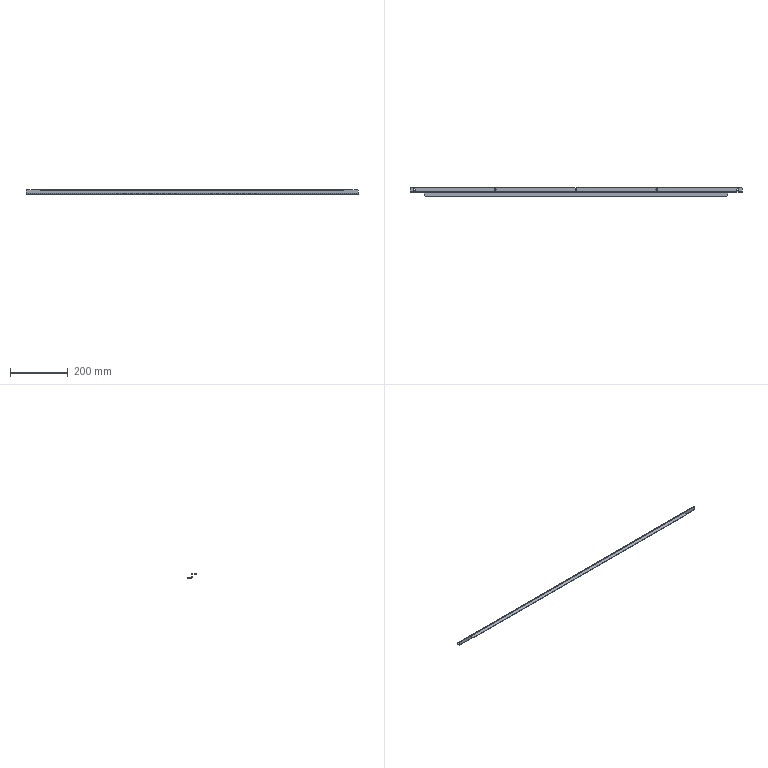Part | NX | features solid 2 | 1 solid | 38 faces | box 1150 x 30.5 x 15 mm | volume 70285 mm3 | plane 24 | cylinder 14 | commonest cylinder face diameters 6 x12 3 x2
STEP:
#1=CARTESIAN_POINT('',(-450.,-634.5,86.));
#2=VERTEX_POINT('',#1);
#3=CARTESIAN_POINT('',(-447.,-634.5,89.));
#4=VERTEX_POINT('',#3);
#5=CARTESIAN_POINT('',(-447.,-634.5,89.));
#6=DIRECTION('',(0.7071,0.,0.7071));
#7=VECTOR('',#6,1000.);
#8=LINE('',#5,#7);
#9=EDGE_CURVE('',#2,#4,#8,.T.);
#10=ORIENTED_EDGE('',*,*,#9,.F.);
#11=CARTESIAN_POINT('',(-450.,-636.,86.));
#12=VERTEX_POINT('',#11);
#13=CARTESIAN_POINT('',(-450.,-636.,86.));
#14=DIRECTION('',(0.,1.,0.));
#15=VECTOR('',#14,1000.);
#16=LINE('',#13,#15);
#17=EDGE_CURVE('',#12,#2,#16,.T.);
#18=ORIENTED_EDGE('',*,*,#17,.F.);
#19=CARTESIAN_POINT('',(-447.,-636.,89.));
#20=VERTEX_POINT('',#19);
#21=CARTESIAN_POINT('',(-448.5,-636.,87.5));
#22=DIRECTION('',(-0.7071,0.,-0.7071));
#23=VECTOR('',#22,1000.);
#24=LINE('',#21,#23);
#25=EDGE_CURVE('',#20,#12,#24,.T.);
#26=ORIENTED_EDGE('',*,*,#25,.F.);
#27=CARTESIAN_POINT('',(-447.,-636.,89.));
#28=DIRECTION('',(0.,-1.,0.));
#29=VECTOR('',#28,1000.);
#30=LINE('',#27,#29);
#31=EDGE_CURVE('',#4,#20,#30,.T.);
#32=ORIENTED_EDGE('',*,*,#31,.F.);
#33=EDGE_LOOP('',(#10,#18,#26,#32));
#34=FACE_BOUND('',#33,.T.);
#35=CARTESIAN_POINT('',(-447.,-636.,89.));
#36=DIRECTION('',(-0.7071,0.,0.7071));
#37=DIRECTION('',(0.,1.,0.));
#38=AXIS2_PLACEMENT_3D('',#35,#36,#37);
#39=PLANE('',#38);
#40=ADVANCED_FACE('',(#34),#39,.T.);
#41=CARTESIAN_POINT('',(-447.,-620.,75.5));
#42=VERTEX_POINT('',#41);
#43=CARTESIAN_POINT('',(-450.,-623.,75.5));
#44=VERTEX_POINT('',#43);
#45=CARTESIAN_POINT('',(-450.,-623.,75.5));
#46=DIRECTION('',(-0.7071,-0.7071,0.));
#47=VECTOR('',#46,1000.);
#48=LINE('',#45,#47);
#49=EDGE_CURVE('',#42,#44,#48,.T.);
#50=ORIENTED_EDGE('',*,*,#49,.F.);
#51=CARTESIAN_POINT('',(-447.,-620.,74.));
#52=VERTEX_POINT('',#51);
#53=CARTESIAN_POINT('',(-447.,-620.,74.));
#54=DIRECTION('',(0.,0.,1.));
#55=VECTOR('',#54,1000.);
#56=LINE('',#53,#55);
#57=EDGE_CURVE('',#52,#42,#56,.T.);
#58=ORIENTED_EDGE('',*,*,#57,.F.);
#59=CARTESIAN_POINT('',(-450.,-623.,74.));
#60=VERTEX_POINT('',#59);
#61=CARTESIAN_POINT('',(-456.5,-629.5,74.));
#62=DIRECTION('',(0.7071,0.7071,0.));
#63=VECTOR('',#62,1000.);
#64=LINE('',#61,#63);
#65=EDGE_CURVE('',#60,#52,#64,.T.);
#66=ORIENTED_EDGE('',*,*,#65,.F.);
#67=CARTESIAN_POINT('',(-450.,-623.,74.));
#68=DIRECTION('',(0.,0.,-1.));
#69=VECTOR('',#68,1000.);
#70=LINE('',#67,#69);
#71=EDGE_CURVE('',#44,#60,#70,.T.);
#72=ORIENTED_EDGE('',*,*,#71,.F.);
#73=EDGE_LOOP('',(#50,#58,#66,#72));
#74=FACE_BOUND('',#73,.T.);
#75=CARTESIAN_POINT('',(-450.,-623.,74.));
#76=DIRECTION('',(0.7071,-0.7071,0.));
#77=DIRECTION('',(0.,0.,-1.));
#78=AXIS2_PLACEMENT_3D('',#75,#76,#77);
#79=PLANE('',#78);
#80=ADVANCED_FACE('',(#74),#79,.F.);
#81=CARTESIAN_POINT('',(-400.,-647.5,89.));
#82=VERTEX_POINT('',#81);
#83=CARTESIAN_POINT('',(-397.,-650.5,89.));
#84=VERTEX_POINT('',#83);
#85=CARTESIAN_POINT('',(-147.25,-900.25,89.));
#86=DIRECTION('',(0.7071,-0.7071,0.));
#87=VECTOR('',#86,1000.);
#88=LINE('',#85,#87);
#89=EDGE_CURVE('',#82,#84,#88,.T.);
#90=ORIENTED_EDGE('',*,*,#89,.F.);
#91=CARTESIAN_POINT('',(-400.,-647.5,87.5));
#92=VERTEX_POINT('',#91);
#93=CARTESIAN_POINT('',(-400.,-647.5,89.));
#94=DIRECTION('',(0.,0.,1.));
#95=VECTOR('',#94,1000.);
#96=LINE('',#93,#95);
#97=EDGE_CURVE('',#92,#82,#96,.T.);
#98=ORIENTED_EDGE('',*,*,#97,.F.);
#99=CARTESIAN_POINT('',(-397.,-650.5,87.5));
#100=VERTEX_POINT('',#99);
#101=CARTESIAN_POINT('',(-397.,-650.5,87.5));
#102=DIRECTION('',(-0.7071,0.7071,0.));
#103=VECTOR('',#102,1000.);
#104=LINE('',#101,#103);
#105=EDGE_CURVE('',#100,#92,#104,.T.);
#106=ORIENTED_EDGE('',*,*,#105,.F.);
#107=CARTESIAN_POINT('',(-397.,-650.5,89.));
#108=DIRECTION('',(0.,0.,-1.));
#109=VECTOR('',#108,1000.);
#110=LINE('',#107,#109);
#111=EDGE_CURVE('',#84,#100,#110,.T.);
#112=ORIENTED_EDGE('',*,*,#111,.F.);
#113=EDGE_LOOP('',(#90,#98,#106,#112));
#114=FACE_BOUND('',#113,.T.);
#115=CARTESIAN_POINT('',(-397.,-650.5,89.));
#116=DIRECTION('',(0.7071,0.7071,0.));
#117=DIRECTION('',(0.,0.,-1.));
#118=AXIS2_PLACEMENT_3D('',#115,#116,#117);
#119=PLANE('',#118);
#120=ADVANCED_FACE('',(#114),#119,.F.);
#121=CARTESIAN_POINT('',(700.,-623.,75.5));
#122=VERTEX_POINT('',#121);
#123=CARTESIAN_POINT('',(697.,-620.,75.5));
#124=VERTEX_POINT('',#123);
#125=CARTESIAN_POINT('',(697.,-620.,75.5));
#126=DIRECTION('',(-0.7071,0.7071,0.));
#127=VECTOR('',#126,1000.);
#128=LINE('',#125,#127);
#129=EDGE_CURVE('',#122,#124,#128,.T.);
#130=ORIENTED_EDGE('',*,*,#129,.F.);
#131=CARTESIAN_POINT('',(700.,-623.,74.));
#132=VERTEX_POINT('',#131);
#133=CARTESIAN_POINT('',(700.,-623.,89.));
#134=DIRECTION('',(0.,0.,1.));
#135=VECTOR('',#134,1000.);
#136=LINE('',#133,#135);
#137=EDGE_CURVE('',#132,#122,#136,.T.);
#138=ORIENTED_EDGE('',*,*,#137,.F.);
#139=CARTESIAN_POINT('',(697.,-620.,74.));
#140=VERTEX_POINT('',#139);
#141=CARTESIAN_POINT('',(131.5,-54.5,74.));
#142=DIRECTION('',(0.7071,-0.7071,0.));
#143=VECTOR('',#142,1000.);
#144=LINE('',#141,#143);
#145=EDGE_CURVE('',#140,#132,#144,.T.);
#146=ORIENTED_EDGE('',*,*,#145,.F.);
#147=CARTESIAN_POINT('',(697.,-620.,74.));
#148=DIRECTION('',(0.,0.,-1.));
#149=VECTOR('',#148,1000.);
#150=LINE('',#147,#149);
#151=EDGE_CURVE('',#124,#140,#150,.T.);
#152=ORIENTED_EDGE('',*,*,#151,.F.);
#153=EDGE_LOOP('',(#130,#138,#146,#152));
#154=FACE_BOUND('',#153,.T.);
#155=CARTESIAN_POINT('',(697.,-620.,74.));
#156=DIRECTION('',(0.7071,0.7071,0.));
#157=DIRECTION('',(0.,0.,-1.));
#158=AXIS2_PLACEMENT_3D('',#155,#156,#157);
#159=PLANE('',#158);
#160=ADVANCED_FACE('',(#154),#159,.T.);
#161=CARTESIAN_POINT('',(697.,-634.5,89.));
#162=VERTEX_POINT('',#161);
#163=CARTESIAN_POINT('',(700.,-634.5,86.));
#164=VERTEX_POINT('',#163);
#165=CARTESIAN_POINT('',(700.,-634.5,86.));
#166=DIRECTION('',(0.7071,0.,-0.7071));
#167=VECTOR('',#166,1000.);
#168=LINE('',#165,#167);
#169=EDGE_CURVE('',#162,#164,#168,.T.);
#170=ORIENTED_EDGE('',*,*,#169,.F.);
#171=CARTESIAN_POINT('',(697.,-636.,89.));
#172=VERTEX_POINT('',#171);
#173=CARTESIAN_POINT('',(697.,-636.,89.));
#174=DIRECTION('',(0.,1.,0.));
#175=VECTOR('',#174,1000.);
#176=LINE('',#173,#175);
#177=EDGE_CURVE('',#172,#162,#176,.T.);
#178=ORIENTED_EDGE('',*,*,#177,.F.);
#179=CARTESIAN_POINT('',(700.,-636.,86.));
#180=VERTEX_POINT('',#179);
#181=CARTESIAN_POINT('',(123.5,-636.,662.5));
#182=DIRECTION('',(-0.7071,0.,0.7071));
#183=VECTOR('',#182,1000.);
#184=LINE('',#181,#183);
#185=EDGE_CURVE('',#180,#172,#184,.T.);
#186=ORIENTED_EDGE('',*,*,#185,.F.);
#187=CARTESIAN_POINT('',(700.,-636.,86.));
#188=DIRECTION('',(0.,-1.,0.));
#189=VECTOR('',#188,1000.);
#190=LINE('',#187,#189);
#191=EDGE_CURVE('',#164,#180,#190,.T.);
#192=ORIENTED_EDGE('',*,*,#191,.F.);
#193=EDGE_LOOP('',(#170,#178,#186,#192));
#194=FACE_BOUND('',#193,.T.);
#195=CARTESIAN_POINT('',(700.,-636.,86.));
#196=DIRECTION('',(-0.7071,0.,-0.7071));
#197=DIRECTION('',(-0.7071,0.,0.7071));
#198=AXIS2_PLACEMENT_3D('',#195,#196,#197);
#199=PLANE('',#198);
#200=ADVANCED_FACE('',(#194),#199,.F.);
#201=CARTESIAN_POINT('',(647.,-650.5,89.));
#202=VERTEX_POINT('',#201);
#203=CARTESIAN_POINT('',(650.,-647.5,89.));
#204=VERTEX_POINT('',#203);
#205=CARTESIAN_POINT('',(397.25,-900.25,89.));
#206=DIRECTION('',(0.7071,0.7071,0.));
#207=VECTOR('',#206,1000.);
#208=LINE('',#205,#207);
#209=EDGE_CURVE('',#202,#204,#208,.T.);
#210=ORIENTED_EDGE('',*,*,#209,.F.);
#211=CARTESIAN_POINT('',(647.,-650.5,87.5));
#212=VERTEX_POINT('',#211);
#213=CARTESIAN_POINT('',(647.,-650.5,89.));
#214=DIRECTION('',(0.,0.,1.));
#215=VECTOR('',#214,1000.);
#216=LINE('',#213,#215);
#217=EDGE_CURVE('',#212,#202,#216,.T.);
#218=ORIENTED_EDGE('',*,*,#217,.F.);
#219=CARTESIAN_POINT('',(650.,-647.5,87.5));
#220=VERTEX_POINT('',#219);
#221=CARTESIAN_POINT('',(650.,-647.5,87.5));
#222=DIRECTION('',(-0.7071,-0.7071,0.));
#223=VECTOR('',#222,1000.);
#224=LINE('',#221,#223);
#225=EDGE_CURVE('',#220,#212,#224,.T.);
#226=ORIENTED_EDGE('',*,*,#225,.F.);
#227=CARTESIAN_POINT('',(650.,-647.5,89.));
#228=DIRECTION('',(0.,0.,-1.));
#229=VECTOR('',#228,1000.);
#230=LINE('',#227,#229);
#231=EDGE_CURVE('',#204,#220,#230,.T.);
#232=ORIENTED_EDGE('',*,*,#231,.F.);
#233=EDGE_LOOP('',(#210,#218,#226,#232));
#234=FACE_BOUND('',#233,.T.);
#235=CARTESIAN_POINT('',(650.,-647.5,89.));
#236=DIRECTION('',(-0.7071,0.7071,0.));
#237=DIRECTION('',(0.,0.,1.));
#238=AXIS2_PLACEMENT_3D('',#235,#236,#237);
#239=PLANE('',#238);
#240=ADVANCED_FACE('',(#234),#239,.F.);
#241=CARTESIAN_POINT('',(685.,-630.,74.));
#242=VERTEX_POINT('',#241);
#243=CARTESIAN_POINT('',(685.,-630.,75.5));
#244=VERTEX_POINT('',#243);
#245=CARTESIAN_POINT('',(685.,-630.,-1075.002));
#246=DIRECTION('',(0.,0.,1.));
#247=VECTOR('',#246,1000.);
#248=LINE('',#245,#247);
#249=EDGE_CURVE('',#242,#244,#248,.T.);
#250=ORIENTED_EDGE('',*,*,#249,.F.);
#251=CARTESIAN_POINT('',(685.,-624.,74.));
#252=VERTEX_POINT('',#251);
#253=CARTESIAN_POINT('',(685.,-627.,74.));
#254=DIRECTION('',(0.,0.,-1.));
#255=DIRECTION('',(0.,-1.,0.));
#256=AXIS2_PLACEMENT_3D('',#253,#254,#255);
#257=CIRCLE('',#256,3.);
#258=EDGE_CURVE('',#242,#252,#257,.T.);
#259=ORIENTED_EDGE('',*,*,#258,.T.);
#260=CARTESIAN_POINT('',(685.,-624.,75.5));
#261=VERTEX_POINT('',#260);
#262=CARTESIAN_POINT('',(685.,-624.,-1075.002));
#263=DIRECTION('',(0.,0.,1.));
#264=VECTOR('',#263,1000.);
#265=LINE('',#262,#264);
#266=EDGE_CURVE('',#261,#252,#265,.F.);
#267=ORIENTED_EDGE('',*,*,#266,.F.);
#268=CARTESIAN_POINT('',(685.,-627.,75.5));
#269=DIRECTION('',(0.,0.,1.));
#270=DIRECTION('',(1.,0.,0.));
#271=AXIS2_PLACEMENT_3D('',#268,#269,#270);
#272=CIRCLE('',#271,3.);
#273=EDGE_CURVE('',#261,#244,#272,.T.);
#274=ORIENTED_EDGE('',*,*,#273,.T.);
#275=EDGE_LOOP('',(#250,#259,#267,#274));
#276=FACE_BOUND('',#275,.T.);
#277=CARTESIAN_POINT('',(685.,-627.,-1075.002));
#278=DIRECTION('',(0.,0.,1.));
#279=DIRECTION('',(0.,1.,0.));
#280=AXIS2_PLACEMENT_3D('',#277,#278,#279);
#281=CYLINDRICAL_SURFACE('',#280,3.);
#282=ADVANCED_FACE('',(#276),#281,.F.);
#283=CARTESIAN_POINT('',(405.,-630.,75.5));
#284=VERTEX_POINT('',#283);
#285=CARTESIAN_POINT('',(405.,-630.,74.));
#286=VERTEX_POINT('',#285);
#287=CARTESIAN_POINT('',(405.,-630.,-1075.002));
#288=DIRECTION('',(0.,0.,1.));
#289=VECTOR('',#288,1000.);
#290=LINE('',#287,#289);
#291=EDGE_CURVE('',#284,#286,#290,.F.);
#292=ORIENTED_EDGE('',*,*,#291,.T.);
#293=CARTESIAN_POINT('',(405.,-624.,74.));
#294=VERTEX_POINT('',#293);
#295=CARTESIAN_POINT('',(405.,-627.,74.));
#296=DIRECTION('',(0.,0.,-1.));
#297=DIRECTION('',(0.,-1.,0.));
#298=AXIS2_PLACEMENT_3D('',#295,#296,#297);
#299=CIRCLE('',#298,3.);
#300=EDGE_CURVE('',#286,#294,#299,.T.);
#301=ORIENTED_EDGE('',*,*,#300,.T.);
#302=CARTESIAN_POINT('',(405.,-624.,75.5));
#303=VERTEX_POINT('',#302);
#304=CARTESIAN_POINT('',(405.,-624.,-1075.002));
#305=DIRECTION('',(0.,0.,1.));
#306=VECTOR('',#305,1000.);
#307=LINE('',#304,#306);
#308=EDGE_CURVE('',#294,#303,#307,.T.);
#309=ORIENTED_EDGE('',*,*,#308,.T.);
#310=CARTESIAN_POINT('',(405.,-627.,75.5));
#311=DIRECTION('',(0.,0.,1.));
#312=DIRECTION('',(1.,0.,0.));
#313=AXIS2_PLACEMENT_3D('',#310,#311,#312);
#314=CIRCLE('',#313,3.);
#315=EDGE_CURVE('',#303,#284,#314,.T.);
#316=ORIENTED_EDGE('',*,*,#315,.T.);
#317=EDGE_LOOP('',(#292,#301,#309,#316));
#318=FACE_BOUND('',#317,.T.);
#319=CARTESIAN_POINT('',(405.,-627.,-1075.002));
#320=DIRECTION('',(0.,0.,1.));
#321=DIRECTION('',(0.,1.,0.));
#322=AXIS2_PLACEMENT_3D('',#319,#320,#321);
#323=CYLINDRICAL_SURFACE('',#322,3.);
#324=ADVANCED_FACE('',(#318),#323,.F.);
#325=CARTESIAN_POINT('',(125.,-630.,75.5));
#326=VERTEX_POINT('',#325);
#327=CARTESIAN_POINT('',(125.,-630.,74.));
#328=VERTEX_POINT('',#327);
#329=CARTESIAN_POINT('',(125.,-630.,-1075.002));
#330=DIRECTION('',(0.,0.,1.));
#331=VECTOR('',#330,1000.);
#332=LINE('',#329,#331);
#333=EDGE_CURVE('',#326,#328,#332,.F.);
#334=ORIENTED_EDGE('',*,*,#333,.T.);
#335=CARTESIAN_POINT('',(125.,-624.,74.));
#336=VERTEX_POINT('',#335);
#337=CARTESIAN_POINT('',(125.,-627.,74.));
#338=DIRECTION('',(0.,0.,-1.));
#339=DIRECTION('',(0.,-1.,0.));
#340=AXIS2_PLACEMENT_3D('',#337,#338,#339);
#341=CIRCLE('',#340,3.);
#342=EDGE_CURVE('',#328,#336,#341,.T.);
#343=ORIENTED_EDGE('',*,*,#342,.T.);
#344=CARTESIAN_POINT('',(125.,-624.,75.5));
#345=VERTEX_POINT('',#344);
#346=CARTESIAN_POINT('',(125.,-624.,-1075.002));
#347=DIRECTION('',(0.,0.,1.));
#348=VECTOR('',#347,1000.);
#349=LINE('',#346,#348);
#350=EDGE_CURVE('',#336,#345,#349,.T.);
#351=ORIENTED_EDGE('',*,*,#350,.T.);
#352=CARTESIAN_POINT('',(125.,-627.,75.5));
#353=DIRECTION('',(0.,0.,1.));
#354=DIRECTION('',(1.,0.,0.));
#355=AXIS2_PLACEMENT_3D('',#352,#353,#354);
#356=CIRCLE('',#355,3.);
#357=EDGE_CURVE('',#345,#326,#356,.T.);
#358=ORIENTED_EDGE('',*,*,#357,.T.);
#359=EDGE_LOOP('',(#334,#343,#351,#358));
#360=FACE_BOUND('',#359,.T.);
#361=CARTESIAN_POINT('',(125.,-627.,-1075.002));
#362=DIRECTION('',(0.,0.,1.));
#363=DIRECTION('',(0.,1.,0.));
#364=AXIS2_PLACEMENT_3D('',#361,#362,#363);
#365=CYLINDRICAL_SURFACE('',#364,3.);
#366=ADVANCED_FACE('',(#360),#365,.F.);
#367=CARTESIAN_POINT('',(-155.,-630.,74.));
#368=VERTEX_POINT('',#367);
#369=CARTESIAN_POINT('',(-155.,-630.,75.5));
#370=VERTEX_POINT('',#369);
#371=CARTESIAN_POINT('',(-155.,-630.,-1075.002));
#372=DIRECTION('',(0.,0.,1.));
#373=VECTOR('',#372,1000.);
#374=LINE('',#371,#373);
#375=EDGE_CURVE('',#368,#370,#374,.T.);
#376=ORIENTED_EDGE('',*,*,#375,.F.);
#377=CARTESIAN_POINT('',(-155.,-624.,74.));
#378=VERTEX_POINT('',#377);
#379=CARTESIAN_POINT('',(-155.,-627.,74.));
#380=DIRECTION('',(0.,0.,-1.));
#381=DIRECTION('',(0.,-1.,0.));
#382=AXIS2_PLACEMENT_3D('',#379,#380,#381);
#383=CIRCLE('',#382,3.);
#384=EDGE_CURVE('',#368,#378,#383,.T.);
#385=ORIENTED_EDGE('',*,*,#384,.T.);
#386=CARTESIAN_POINT('',(-155.,-624.,75.5));
#387=VERTEX_POINT('',#386);
#388=CARTESIAN_POINT('',(-155.,-624.,-1075.002));
#389=DIRECTION('',(0.,0.,1.));
#390=VECTOR('',#389,1000.);
#391=LINE('',#388,#390);
#392=EDGE_CURVE('',#387,#378,#391,.F.);
#393=ORIENTED_EDGE('',*,*,#392,.F.);
#394=CARTESIAN_POINT('',(-155.,-627.,75.5));
#395=DIRECTION('',(0.,0.,1.));
#396=DIRECTION('',(1.,0.,0.));
#397=AXIS2_PLACEMENT_3D('',#394,#395,#396);
#398=CIRCLE('',#397,3.);
#399=EDGE_CURVE('',#387,#370,#398,.T.);
#400=ORIENTED_EDGE('',*,*,#399,.T.);
#401=EDGE_LOOP('',(#376,#385,#393,#400));
#402=FACE_BOUND('',#401,.T.);
#403=CARTESIAN_POINT('',(-155.,-627.,-1075.002));
#404=DIRECTION('',(0.,0.,1.));
#405=DIRECTION('',(0.,1.,0.));
#406=AXIS2_PLACEMENT_3D('',#403,#404,#405);
#407=CYLINDRICAL_SURFACE('',#406,3.);
#408=ADVANCED_FACE('',(#402),#407,.F.);
#409=CARTESIAN_POINT('',(-435.,-630.,74.));
#410=VERTEX_POINT('',#409);
#411=CARTESIAN_POINT('',(-435.,-630.,75.5));
#412=VERTEX_POINT('',#411);
#413=CARTESIAN_POINT('',(-435.,-630.,-1075.002));
#414=DIRECTION('',(0.,0.,1.));
#415=VECTOR('',#414,1000.);
#416=LINE('',#413,#415);
#417=EDGE_CURVE('',#410,#412,#416,.T.);
#418=ORIENTED_EDGE('',*,*,#417,.F.);
#419=CARTESIAN_POINT('',(-435.,-624.,74.));
#420=VERTEX_POINT('',#419);
#421=CARTESIAN_POINT('',(-435.,-627.,74.));
#422=DIRECTION('',(0.,0.,-1.));
#423=DIRECTION('',(0.,-1.,0.));
#424=AXIS2_PLACEMENT_3D('',#421,#422,#423);
#425=CIRCLE('',#424,3.);
#426=EDGE_CURVE('',#410,#420,#425,.T.);
#427=ORIENTED_EDGE('',*,*,#426,.T.);
#428=CARTESIAN_POINT('',(-435.,-624.,75.5));
#429=VERTEX_POINT('',#428);
#430=CARTESIAN_POINT('',(-435.,-624.,-1075.002));
#431=DIRECTION('',(0.,0.,1.));
#432=VECTOR('',#431,1000.);
#433=LINE('',#430,#432);
#434=EDGE_CURVE('',#429,#420,#433,.F.);
#435=ORIENTED_EDGE('',*,*,#434,.F.);
#436=CARTESIAN_POINT('',(-435.,-627.,75.5));
#437=DIRECTION('',(0.,0.,1.));
#438=DIRECTION('',(1.,0.,0.));
#439=AXIS2_PLACEMENT_3D('',#436,#437,#438);
#440=CIRCLE('',#439,3.);
#441=EDGE_CURVE('',#429,#412,#440,.T.);
#442=ORIENTED_EDGE('',*,*,#441,.T.);
#443=EDGE_LOOP('',(#418,#427,#435,#442));
#444=FACE_BOUND('',#443,.T.);
#445=CARTESIAN_POINT('',(-435.,-627.,-1075.002));
#446=DIRECTION('',(0.,0.,1.));
#447=DIRECTION('',(0.,1.,0.));
#448=AXIS2_PLACEMENT_3D('',#445,#446,#447);
#449=CYLINDRICAL_SURFACE('',#448,3.);
#450=ADVANCED_FACE('',(#444),#449,.F.);
#451=CARTESIAN_POINT('',(-400.,-636.,86.));
#452=VERTEX_POINT('',#451);
#453=CARTESIAN_POINT('',(650.,-636.,86.));
#454=VERTEX_POINT('',#453);
#455=CARTESIAN_POINT('',(-400.,-636.,86.));
#456=DIRECTION('',(1.,0.,0.));
#457=VECTOR('',#456,1000.);
#458=LINE('',#455,#457);
#459=EDGE_CURVE('',#452,#454,#458,.T.);
#460=ORIENTED_EDGE('',*,*,#459,.T.);
#461=CARTESIAN_POINT('',(650.,-637.5,87.5));
#462=VERTEX_POINT('',#461);
#463=CARTESIAN_POINT('',(650.,-637.5,86.));
#464=DIRECTION('',(-1.,0.,0.));
#465=DIRECTION('',(0.,0.,-1.));
#466=AXIS2_PLACEMENT_3D('',#463,#464,#465);
#467=CIRCLE('',#466,1.5);
#468=EDGE_CURVE('',#462,#454,#467,.T.);
#469=ORIENTED_EDGE('',*,*,#468,.F.);
#470=CARTESIAN_POINT('',(-400.,-637.5,87.5));
#471=VERTEX_POINT('',#470);
#472=CARTESIAN_POINT('',(650.,-637.5,87.5));
#473=DIRECTION('',(-1.,0.,0.));
#474=VECTOR('',#473,1000.);
#475=LINE('',#472,#474);
#476=EDGE_CURVE('',#462,#471,#475,.T.);
#477=ORIENTED_EDGE('',*,*,#476,.T.);
#478=CARTESIAN_POINT('',(-400.,-637.5,86.));
#479=DIRECTION('',(-1.,0.,0.));
#480=DIRECTION('',(0.,0.,-1.));
#481=AXIS2_PLACEMENT_3D('',#478,#479,#480);
#482=CIRCLE('',#481,1.5);
#483=EDGE_CURVE('',#471,#452,#482,.T.);
#484=ORIENTED_EDGE('',*,*,#483,.T.);
#485=EDGE_LOOP('',(#460,#469,#477,#484));
#486=FACE_BOUND('',#485,.T.);
#487=CARTESIAN_POINT('',(-400.,-637.5,86.));
#488=DIRECTION('',(1.,0.,0.));
#489=DIRECTION('',(0.,-1.,0.));
#490=AXIS2_PLACEMENT_3D('',#487,#488,#489);
#491=CYLINDRICAL_SURFACE('',#490,1.5);
#492=ADVANCED_FACE('',(#486),#491,.F.);
#493=CARTESIAN_POINT('',(-400.,-634.5,86.));
#494=VERTEX_POINT('',#493);
#495=CARTESIAN_POINT('',(650.,-634.5,86.));
#496=VERTEX_POINT('',#495);
#497=CARTESIAN_POINT('',(-400.,-634.5,86.));
#498=DIRECTION('',(1.,0.,0.));
#499=VECTOR('',#498,1000.);
#500=LINE('',#497,#499);
#501=EDGE_CURVE('',#494,#496,#500,.T.);
#502=ORIENTED_EDGE('',*,*,#501,.F.);
#503=CARTESIAN_POINT('',(-400.,-637.5,89.));
#504=VERTEX_POINT('',#503);
#505=CARTESIAN_POINT('',(-400.,-637.5,86.));
#506=DIRECTION('',(-1.,0.,0.));
#507=DIRECTION('',(0.,-1.,0.));
#508=AXIS2_PLACEMENT_3D('',#505,#506,#507);
#509=CIRCLE('',#508,3.);
#510=EDGE_CURVE('',#504,#494,#509,.T.);
#511=ORIENTED_EDGE('',*,*,#510,.F.);
#512=CARTESIAN_POINT('',(650.,-637.5,89.));
#513=VERTEX_POINT('',#512);
#514=CARTESIAN_POINT('',(650.,-637.5,89.));
#515=DIRECTION('',(-1.,0.,0.));
#516=VECTOR('',#515,1000.);
#517=LINE('',#514,#516);
#518=EDGE_CURVE('',#513,#504,#517,.T.);
#519=ORIENTED_EDGE('',*,*,#518,.F.);
#520=CARTESIAN_POINT('',(650.,-637.5,86.));
#521=DIRECTION('',(-1.,0.,0.));
#522=DIRECTION('',(0.,-1.,0.));
#523=AXIS2_PLACEMENT_3D('',#520,#521,#522);
#524=CIRCLE('',#523,3.);
#525=EDGE_CURVE('',#513,#496,#524,.T.);
#526=ORIENTED_EDGE('',*,*,#525,.T.);
#527=EDGE_LOOP('',(#502,#511,#519,#526));
#528=FACE_BOUND('',#527,.T.);
#529=CARTESIAN_POINT('',(-400.,-637.5,86.));
#530=DIRECTION('',(1.,0.,0.));
#531=DIRECTION('',(0.,-1.,0.));
#532=AXIS2_PLACEMENT_3D('',#529,#530,#531);
#533=CYLINDRICAL_SURFACE('',#532,3.);
#534=ADVANCED_FACE('',(#528),#533,.T.);
#535=CARTESIAN_POINT('',(-400.,-650.5,87.5));
#536=DIRECTION('',(1.,0.,0.));
#537=VECTOR('',#536,1000.);
#538=LINE('',#535,#537);
#539=EDGE_CURVE('',#100,#212,#538,.T.);
#540=ORIENTED_EDGE('',*,*,#539,.T.);
#541=ORIENTED_EDGE('',*,*,#217,.T.);
#542=CARTESIAN_POINT('',(-400.,-650.5,89.));
#543=DIRECTION('',(1.,0.,0.));
#544=VECTOR('',#543,1000.);
#545=LINE('',#542,#544);
#546=EDGE_CURVE('',#84,#202,#545,.T.);
#547=ORIENTED_EDGE('',*,*,#546,.F.);
#548=ORIENTED_EDGE('',*,*,#111,.T.);
#549=EDGE_LOOP('',(#540,#541,#547,#548));
#550=FACE_BOUND('',#549,.T.);
#551=CARTESIAN_POINT('',(-400.,-650.5,89.));
#552=DIRECTION('',(0.,1.,0.));
#553=DIRECTION('',(1.,0.,0.));
#554=AXIS2_PLACEMENT_3D('',#551,#552,#553);
#555=PLANE('',#554);
#556=ADVANCED_FACE('',(#550),#555,.F.);
#557=CARTESIAN_POINT('',(650.,-635.851,87.5));
#558=DIRECTION('',(0.,1.,0.));
#559=VECTOR('',#558,1000.);
#560=LINE('',#557,#559);
#561=EDGE_CURVE('',#220,#462,#560,.T.);
#562=ORIENTED_EDGE('',*,*,#561,.F.);
#563=ORIENTED_EDGE('',*,*,#225,.T.);
#564=ORIENTED_EDGE('',*,*,#539,.F.);
#565=ORIENTED_EDGE('',*,*,#105,.T.);
#566=CARTESIAN_POINT('',(-400.,-635.851,87.5));
#567=DIRECTION('',(0.,-1.,0.));
#568=VECTOR('',#567,1000.);
#569=LINE('',#566,#568);
#570=EDGE_CURVE('',#471,#92,#569,.T.);
#571=ORIENTED_EDGE('',*,*,#570,.F.);
#572=ORIENTED_EDGE('',*,*,#476,.F.);
#573=EDGE_LOOP('',(#562,#563,#564,#565,#571,#572));
#574=FACE_BOUND('',#573,.T.);
#575=CARTESIAN_POINT('',(125.,-628.,87.5));
#576=DIRECTION('',(0.,0.,1.));
#577=DIRECTION('',(1.,0.,0.));
#578=AXIS2_PLACEMENT_3D('',#575,#576,#577);
#579=PLANE('',#578);
#580=ADVANCED_FACE('',(#574),#579,.F.);
#581=ORIENTED_EDGE('',*,*,#546,.T.);
#582=ORIENTED_EDGE('',*,*,#209,.T.);
#583=CARTESIAN_POINT('',(650.,-635.851,89.));
#584=DIRECTION('',(0.,1.,0.));
#585=VECTOR('',#584,1000.);
#586=LINE('',#583,#585);
#587=EDGE_CURVE('',#204,#513,#586,.T.);
#588=ORIENTED_EDGE('',*,*,#587,.T.);
#589=ORIENTED_EDGE('',*,*,#518,.T.);
#590=CARTESIAN_POINT('',(-400.,-635.851,89.));
#591=DIRECTION('',(0.,-1.,0.));
#592=VECTOR('',#591,1000.);
#593=LINE('',#590,#592);
#594=EDGE_CURVE('',#504,#82,#593,.T.);
#595=ORIENTED_EDGE('',*,*,#594,.T.);
#596=ORIENTED_EDGE('',*,*,#89,.T.);
#597=EDGE_LOOP('',(#581,#582,#588,#589,#595,#596));
#598=FACE_BOUND('',#597,.T.);
#599=CARTESIAN_POINT('',(125.,-628.,89.));
#600=DIRECTION('',(0.,0.,1.));
#601=DIRECTION('',(1.,0.,0.));
#602=AXIS2_PLACEMENT_3D('',#599,#600,#601);
#603=PLANE('',#602);
#604=ADVANCED_FACE('',(#598),#603,.T.);
#605=CARTESIAN_POINT('',(650.1,-636.,85.9));
#606=VERTEX_POINT('',#605);
#607=CARTESIAN_POINT('',(650.1,-634.5,85.9));
#608=VERTEX_POINT('',#607);
#609=CARTESIAN_POINT('',(650.1,-634.5,85.9));
#610=DIRECTION('',(0.,1.,0.));
#611=VECTOR('',#610,1000.);
#612=LINE('',#609,#611);
#613=EDGE_CURVE('',#606,#608,#612,.T.);
#614=ORIENTED_EDGE('',*,*,#613,.T.);
#615=CARTESIAN_POINT('',(650.,-634.5,85.9));
#616=VERTEX_POINT('',#615);
#617=CARTESIAN_POINT('',(650.1,-634.5,85.9));
#618=DIRECTION('',(1.,0.,0.));
#619=VECTOR('',#618,1000.);
#620=LINE('',#617,#619);
#621=EDGE_CURVE('',#616,#608,#620,.T.);
#622=ORIENTED_EDGE('',*,*,#621,.F.);
#623=CARTESIAN_POINT('',(650.,-636.,85.9));
#624=VERTEX_POINT('',#623);
#625=CARTESIAN_POINT('',(650.,-634.5,85.9));
#626=DIRECTION('',(0.,1.,0.));
#627=VECTOR('',#626,1000.);
#628=LINE('',#625,#627);
#629=EDGE_CURVE('',#624,#616,#628,.T.);
#630=ORIENTED_EDGE('',*,*,#629,.F.);
#631=CARTESIAN_POINT('',(650.,-636.,85.9));
#632=DIRECTION('',(1.,0.,0.));
#633=VECTOR('',#632,1000.);
#634=LINE('',#631,#633);
#635=EDGE_CURVE('',#624,#606,#634,.T.);
#636=ORIENTED_EDGE('',*,*,#635,.T.);
#637=EDGE_LOOP('',(#614,#622,#630,#636));
#638=FACE_BOUND('',#637,.T.);
#639=CARTESIAN_POINT('',(650.1,-634.5,85.9));
#640=DIRECTION('',(0.,0.,-1.));
#641=DIRECTION('',(-1.,0.,0.));
#642=AXIS2_PLACEMENT_3D('',#639,#640,#641);
#643=PLANE('',#642);
#644=ADVANCED_FACE('',(#638),#643,.F.);
#645=CARTESIAN_POINT('',(650.1,-636.,89.));
#646=VERTEX_POINT('',#645);
#647=CARTESIAN_POINT('',(650.1,-634.5,89.));
#648=VERTEX_POINT('',#647);
#649=CARTESIAN_POINT('',(650.1,-634.5,89.));
#650=DIRECTION('',(0.,1.,0.));
#651=VECTOR('',#650,1000.);
#652=LINE('',#649,#651);
#653=EDGE_CURVE('',#646,#648,#652,.T.);
#654=ORIENTED_EDGE('',*,*,#653,.T.);
#655=CARTESIAN_POINT('',(650.1,-634.5,89.));
#656=DIRECTION('',(0.,0.,1.));
#657=VECTOR('',#656,1000.);
#658=LINE('',#655,#657);
#659=EDGE_CURVE('',#608,#648,#658,.T.);
#660=ORIENTED_EDGE('',*,*,#659,.F.);
#661=ORIENTED_EDGE('',*,*,#613,.F.);
#662=CARTESIAN_POINT('',(650.1,-636.,85.9));
#663=DIRECTION('',(0.,0.,1.));
#664=VECTOR('',#663,1000.);
#665=LINE('',#662,#664);
#666=EDGE_CURVE('',#606,#646,#665,.T.);
#667=ORIENTED_EDGE('',*,*,#666,.T.);
#668=EDGE_LOOP('',(#654,#660,#661,#667));
#669=FACE_BOUND('',#668,.T.);
#670=CARTESIAN_POINT('',(650.1,-634.5,89.));
#671=DIRECTION('',(1.,0.,0.));
#672=DIRECTION('',(0.,-1.,0.));
#673=AXIS2_PLACEMENT_3D('',#670,#671,#672);
#674=PLANE('',#673);
#675=ADVANCED_FACE('',(#669),#674,.F.);
#676=CARTESIAN_POINT('',(-400.,-636.,85.9));
#677=VERTEX_POINT('',#676);
#678=CARTESIAN_POINT('',(-400.1,-636.,85.9));
#679=VERTEX_POINT('',#678);
#680=CARTESIAN_POINT('',(-400.,-636.,85.9));
#681=DIRECTION('',(-1.,0.,0.));
#682=VECTOR('',#681,1000.);
#683=LINE('',#680,#682);
#684=EDGE_CURVE('',#677,#679,#683,.T.);
#685=ORIENTED_EDGE('',*,*,#684,.F.);
#686=CARTESIAN_POINT('',(-400.,-634.5,85.9));
#687=VERTEX_POINT('',#686);
#688=CARTESIAN_POINT('',(-400.,-634.5,85.9));
#689=DIRECTION('',(0.,1.,0.));
#690=VECTOR('',#689,1000.);
#691=LINE('',#688,#690);
#692=EDGE_CURVE('',#677,#687,#691,.T.);
#693=ORIENTED_EDGE('',*,*,#692,.T.);
#694=CARTESIAN_POINT('',(-400.1,-634.5,85.9));
#695=VERTEX_POINT('',#694);
#696=CARTESIAN_POINT('',(-400.1,-634.5,85.9));
#697=DIRECTION('',(-1.,0.,0.));
#698=VECTOR('',#697,1000.);
#699=LINE('',#696,#698);
#700=EDGE_CURVE('',#687,#695,#699,.T.);
#701=ORIENTED_EDGE('',*,*,#700,.T.);
#702=CARTESIAN_POINT('',(-400.1,-634.5,85.9));
#703=DIRECTION('',(0.,1.,0.));
#704=VECTOR('',#703,1000.);
#705=LINE('',#702,#704);
#706=EDGE_CURVE('',#679,#695,#705,.T.);
#707=ORIENTED_EDGE('',*,*,#706,.F.);
#708=EDGE_LOOP('',(#685,#693,#701,#707));
#709=FACE_BOUND('',#708,.T.);
#710=CARTESIAN_POINT('',(-400.1,-634.5,85.9));
#711=DIRECTION('',(0.,0.,-1.));
#712=DIRECTION('',(-1.,0.,0.));
#713=AXIS2_PLACEMENT_3D('',#710,#711,#712);
#714=PLANE('',#713);
#715=ADVANCED_FACE('',(#709),#714,.F.);
#716=ORIENTED_EDGE('',*,*,#706,.T.);
#717=CARTESIAN_POINT('',(-400.1,-634.5,89.));
#718=VERTEX_POINT('',#717);
#719=CARTESIAN_POINT('',(-400.1,-634.5,89.));
#720=DIRECTION('',(0.,0.,1.));
#721=VECTOR('',#720,1000.);
#722=LINE('',#719,#721);
#723=EDGE_CURVE('',#695,#718,#722,.T.);
#724=ORIENTED_EDGE('',*,*,#723,.T.);
#725=CARTESIAN_POINT('',(-400.1,-636.,89.));
#726=VERTEX_POINT('',#725);
#727=CARTESIAN_POINT('',(-400.1,-634.5,89.));
#728=DIRECTION('',(0.,1.,0.));
#729=VECTOR('',#728,1000.);
#730=LINE('',#727,#729);
#731=EDGE_CURVE('',#726,#718,#730,.T.);
#732=ORIENTED_EDGE('',*,*,#731,.F.);
#733=CARTESIAN_POINT('',(-400.1,-636.,85.9));
#734=DIRECTION('',(0.,0.,1.));
#735=VECTOR('',#734,1000.);
#736=LINE('',#733,#735);
#737=EDGE_CURVE('',#679,#726,#736,.T.);
#738=ORIENTED_EDGE('',*,*,#737,.F.);
#739=EDGE_LOOP('',(#716,#724,#732,#738));
#740=FACE_BOUND('',#739,.T.);
#741=CARTESIAN_POINT('',(-400.1,-634.5,89.));
#742=DIRECTION('',(-1.,0.,0.));
#743=DIRECTION('',(0.,0.,1.));
#744=AXIS2_PLACEMENT_3D('',#741,#742,#743);
#745=PLANE('',#744);
#746=ADVANCED_FACE('',(#740),#745,.F.);
#747=ORIENTED_EDGE('',*,*,#441,.F.);
#748=CARTESIAN_POINT('',(-435.,-627.,75.5));
#749=DIRECTION('',(0.,0.,1.));
#750=DIRECTION('',(1.,0.,0.));
#751=AXIS2_PLACEMENT_3D('',#748,#749,#750);
#752=CIRCLE('',#751,3.);
#753=EDGE_CURVE('',#412,#429,#752,.T.);
#754=ORIENTED_EDGE('',*,*,#753,.F.);
#755=EDGE_LOOP('',(#747,#754));
#756=FACE_BOUND('',#755,.T.);
#757=ORIENTED_EDGE('',*,*,#399,.F.);
#758=CARTESIAN_POINT('',(-155.,-627.,75.5));
#759=DIRECTION('',(0.,0.,1.));
#760=DIRECTION('',(1.,0.,0.));
#761=AXIS2_PLACEMENT_3D('',#758,#759,#760);
#762=CIRCLE('',#761,3.);
#763=EDGE_CURVE('',#370,#387,#762,.T.);
#764=ORIENTED_EDGE('',*,*,#763,.F.);
#765=EDGE_LOOP('',(#757,#764));
#766=FACE_BOUND('',#765,.T.);
#767=ORIENTED_EDGE('',*,*,#357,.F.);
#768=CARTESIAN_POINT('',(125.,-627.,75.5));
#769=DIRECTION('',(0.,0.,1.));
#770=DIRECTION('',(1.,0.,0.));
#771=AXIS2_PLACEMENT_3D('',#768,#769,#770);
#772=CIRCLE('',#771,3.);
#773=EDGE_CURVE('',#326,#345,#772,.T.);
#774=ORIENTED_EDGE('',*,*,#773,.F.);
#775=EDGE_LOOP('',(#767,#774));
#776=FACE_BOUND('',#775,.T.);
#777=ORIENTED_EDGE('',*,*,#315,.F.);
#778=CARTESIAN_POINT('',(405.,-627.,75.5));
#779=DIRECTION('',(0.,0.,1.));
#780=DIRECTION('',(1.,0.,0.));
#781=AXIS2_PLACEMENT_3D('',#778,#779,#780);
#782=CIRCLE('',#781,3.);
#783=EDGE_CURVE('',#284,#303,#782,.T.);
#784=ORIENTED_EDGE('',*,*,#783,.F.);
#785=EDGE_LOOP('',(#777,#784));
#786=FACE_BOUND('',#785,.T.);
#787=ORIENTED_EDGE('',*,*,#273,.F.);
#788=CARTESIAN_POINT('',(685.,-627.,75.5));
#789=DIRECTION('',(0.,0.,1.));
#790=DIRECTION('',(1.,0.,0.));
#791=AXIS2_PLACEMENT_3D('',#788,#789,#790);
#792=CIRCLE('',#791,3.);
#793=EDGE_CURVE('',#244,#261,#792,.T.);
#794=ORIENTED_EDGE('',*,*,#793,.F.);
#795=EDGE_LOOP('',(#787,#794));
#796=FACE_BOUND('',#795,.T.);
#797=CARTESIAN_POINT('',(700.,-633.,75.5));
#798=VERTEX_POINT('',#797);
#799=CARTESIAN_POINT('',(700.,-636.,75.5));
#800=DIRECTION('',(0.,1.,0.));
#801=VECTOR('',#800,1000.);
#802=LINE('',#799,#801);
#803=EDGE_CURVE('',#798,#122,#802,.T.);
#804=ORIENTED_EDGE('',*,*,#803,.T.);
#805=ORIENTED_EDGE('',*,*,#129,.T.);
#806=CARTESIAN_POINT('',(-450.,-620.,75.5));
#807=DIRECTION('',(1.,0.,0.));
#808=VECTOR('',#807,1000.);
#809=LINE('',#806,#808);
#810=EDGE_CURVE('',#42,#124,#809,.T.);
#811=ORIENTED_EDGE('',*,*,#810,.F.);
#812=ORIENTED_EDGE('',*,*,#49,.T.);
#813=CARTESIAN_POINT('',(-450.,-633.,75.5));
#814=VERTEX_POINT('',#813);
#815=CARTESIAN_POINT('',(-450.,-636.,75.5));
#816=DIRECTION('',(0.,1.,0.));
#817=VECTOR('',#816,1000.);
#818=LINE('',#815,#817);
#819=EDGE_CURVE('',#814,#44,#818,.T.);
#820=ORIENTED_EDGE('',*,*,#819,.F.);
#821=CARTESIAN_POINT('',(-450.,-633.,75.5));
#822=DIRECTION('',(1.,0.,0.));
#823=VECTOR('',#822,1000.);
#824=LINE('',#821,#823);
#825=EDGE_CURVE('',#814,#798,#824,.T.);
#826=ORIENTED_EDGE('',*,*,#825,.T.);
#827=EDGE_LOOP('',(#804,#805,#811,#812,#820,#826));
#828=FACE_BOUND('',#827,.T.);
#829=CARTESIAN_POINT('',(-450.,-636.,75.5));
#830=DIRECTION('',(0.,0.,-1.));
#831=DIRECTION('',(-1.,0.,0.));
#832=AXIS2_PLACEMENT_3D('',#829,#830,#831);
#833=PLANE('',#832);
#834=ADVANCED_FACE('',(#756,#766,#776,#786,#796,#828),#833,.F.);
#835=CARTESIAN_POINT('',(700.,-634.5,77.));
#836=VERTEX_POINT('',#835);
#837=CARTESIAN_POINT('',(700.,-633.,77.));
#838=DIRECTION('',(1.,0.,0.));
#839=DIRECTION('',(0.,0.,-1.));
#840=AXIS2_PLACEMENT_3D('',#837,#838,#839);
#841=CIRCLE('',#840,1.5);
#842=EDGE_CURVE('',#836,#798,#841,.T.);
#843=ORIENTED_EDGE('',*,*,#842,.T.);
#844=ORIENTED_EDGE('',*,*,#825,.F.);
#845=CARTESIAN_POINT('',(-450.,-634.5,77.));
#846=VERTEX_POINT('',#845);
#847=CARTESIAN_POINT('',(-450.,-633.,77.));
#848=DIRECTION('',(1.,0.,0.));
#849=DIRECTION('',(0.,0.,-1.));
#850=AXIS2_PLACEMENT_3D('',#847,#848,#849);
#851=CIRCLE('',#850,1.5);
#852=EDGE_CURVE('',#846,#814,#851,.T.);
#853=ORIENTED_EDGE('',*,*,#852,.F.);
#854=CARTESIAN_POINT('',(-450.,-634.5,77.));
#855=DIRECTION('',(1.,0.,0.));
#856=VECTOR('',#855,1000.);
#857=LINE('',#854,#856);
#858=EDGE_CURVE('',#846,#836,#857,.T.);
#859=ORIENTED_EDGE('',*,*,#858,.T.);
#860=EDGE_LOOP('',(#843,#844,#853,#859));
#861=FACE_BOUND('',#860,.T.);
#862=CARTESIAN_POINT('',(-450.,-633.,77.));
#863=DIRECTION('',(1.,0.,0.));
#864=DIRECTION('',(0.,0.,-1.));
#865=AXIS2_PLACEMENT_3D('',#862,#863,#864);
#866=CYLINDRICAL_SURFACE('',#865,1.5);
#867=ADVANCED_FACE('',(#861),#866,.F.);
#868=CARTESIAN_POINT('',(-435.,-627.,74.));
#869=DIRECTION('',(0.,0.,-1.));
#870=DIRECTION('',(0.,-1.,0.));
#871=AXIS2_PLACEMENT_3D('',#868,#869,#870);
#872=CIRCLE('',#871,3.);
#873=EDGE_CURVE('',#420,#410,#872,.T.);
#874=ORIENTED_EDGE('',*,*,#873,.F.);
#875=ORIENTED_EDGE('',*,*,#426,.F.);
#876=EDGE_LOOP('',(#874,#875));
#877=FACE_BOUND('',#876,.T.);
#878=CARTESIAN_POINT('',(-155.,-627.,74.));
#879=DIRECTION('',(0.,0.,-1.));
#880=DIRECTION('',(0.,-1.,0.));
#881=AXIS2_PLACEMENT_3D('',#878,#879,#880);
#882=CIRCLE('',#881,3.);
#883=EDGE_CURVE('',#378,#368,#882,.T.);
#884=ORIENTED_EDGE('',*,*,#883,.F.);
#885=ORIENTED_EDGE('',*,*,#384,.F.);
#886=EDGE_LOOP('',(#884,#885));
#887=FACE_BOUND('',#886,.T.);
#888=CARTESIAN_POINT('',(125.,-627.,74.));
#889=DIRECTION('',(0.,0.,-1.));
#890=DIRECTION('',(0.,-1.,0.));
#891=AXIS2_PLACEMENT_3D('',#888,#889,#890);
#892=CIRCLE('',#891,3.);
#893=EDGE_CURVE('',#336,#328,#892,.T.);
#894=ORIENTED_EDGE('',*,*,#893,.F.);
#895=ORIENTED_EDGE('',*,*,#342,.F.);
#896=EDGE_LOOP('',(#894,#895));
#897=FACE_BOUND('',#896,.T.);
#898=CARTESIAN_POINT('',(405.,-627.,74.));
#899=DIRECTION('',(0.,0.,-1.));
#900=DIRECTION('',(0.,-1.,0.));
#901=AXIS2_PLACEMENT_3D('',#898,#899,#900);
#902=CIRCLE('',#901,3.);
#903=EDGE_CURVE('',#294,#286,#902,.T.);
#904=ORIENTED_EDGE('',*,*,#903,.F.);
#905=ORIENTED_EDGE('',*,*,#300,.F.);
#906=EDGE_LOOP('',(#904,#905));
#907=FACE_BOUND('',#906,.T.);
#908=CARTESIAN_POINT('',(685.,-627.,74.));
#909=DIRECTION('',(0.,0.,-1.));
#910=DIRECTION('',(0.,-1.,0.));
#911=AXIS2_PLACEMENT_3D('',#908,#909,#910);
#912=CIRCLE('',#911,3.);
#913=EDGE_CURVE('',#252,#242,#912,.T.);
#914=ORIENTED_EDGE('',*,*,#913,.F.);
#915=ORIENTED_EDGE('',*,*,#258,.F.);
#916=EDGE_LOOP('',(#914,#915));
#917=FACE_BOUND('',#916,.T.);
#918=CARTESIAN_POINT('',(-450.,-620.,74.));
#919=DIRECTION('',(1.,0.,0.));
#920=VECTOR('',#919,1000.);
#921=LINE('',#918,#920);
#922=EDGE_CURVE('',#52,#140,#921,.T.);
#923=ORIENTED_EDGE('',*,*,#922,.T.);
#924=ORIENTED_EDGE('',*,*,#145,.T.);
#925=CARTESIAN_POINT('',(700.,-633.,74.));
#926=VERTEX_POINT('',#925);
#927=CARTESIAN_POINT('',(700.,-636.,74.));
#928=DIRECTION('',(0.,1.,0.));
#929=VECTOR('',#928,1000.);
#930=LINE('',#927,#929);
#931=EDGE_CURVE('',#926,#132,#930,.T.);
#932=ORIENTED_EDGE('',*,*,#931,.F.);
#933=CARTESIAN_POINT('',(-450.,-633.,74.));
#934=VERTEX_POINT('',#933);
#935=CARTESIAN_POINT('',(-450.,-633.,74.));
#936=DIRECTION('',(1.,0.,0.));
#937=VECTOR('',#936,1000.);
#938=LINE('',#935,#937);
#939=EDGE_CURVE('',#934,#926,#938,.T.);
#940=ORIENTED_EDGE('',*,*,#939,.F.);
#941=CARTESIAN_POINT('',(-450.,-636.,74.));
#942=DIRECTION('',(0.,1.,0.));
#943=VECTOR('',#942,1000.);
#944=LINE('',#941,#943);
#945=EDGE_CURVE('',#934,#60,#944,.T.);
#946=ORIENTED_EDGE('',*,*,#945,.T.);
#947=ORIENTED_EDGE('',*,*,#65,.T.);
#948=EDGE_LOOP('',(#923,#924,#932,#940,#946,#947));
#949=FACE_BOUND('',#948,.T.);
#950=CARTESIAN_POINT('',(-450.,-636.,74.));
#951=DIRECTION('',(0.,0.,-1.));
#952=DIRECTION('',(-1.,0.,0.));
#953=AXIS2_PLACEMENT_3D('',#950,#951,#952);
#954=PLANE('',#953);
#955=ADVANCED_FACE('',(#877,#887,#897,#907,#917,#949),#954,.T.);
#956=CARTESIAN_POINT('',(700.,-636.,77.));
#957=VERTEX_POINT('',#956);
#958=CARTESIAN_POINT('',(700.,-633.,77.));
#959=DIRECTION('',(1.,0.,0.));
#960=DIRECTION('',(0.,0.,1.));
#961=AXIS2_PLACEMENT_3D('',#958,#959,#960);
#962=CIRCLE('',#961,3.);
#963=EDGE_CURVE('',#957,#926,#962,.T.);
#964=ORIENTED_EDGE('',*,*,#963,.F.);
#965=CARTESIAN_POINT('',(-450.,-636.,77.));
#966=VERTEX_POINT('',#965);
#967=CARTESIAN_POINT('',(-450.,-636.,77.));
#968=DIRECTION('',(1.,0.,0.));
#969=VECTOR('',#968,1000.);
#970=LINE('',#967,#969);
#971=EDGE_CURVE('',#966,#957,#970,.T.);
#972=ORIENTED_EDGE('',*,*,#971,.F.);
#973=CARTESIAN_POINT('',(-450.,-633.,77.));
#974=DIRECTION('',(1.,0.,0.));
#975=DIRECTION('',(0.,0.,1.));
#976=AXIS2_PLACEMENT_3D('',#973,#974,#975);
#977=CIRCLE('',#976,3.);
#978=EDGE_CURVE('',#966,#934,#977,.T.);
#979=ORIENTED_EDGE('',*,*,#978,.T.);
#980=ORIENTED_EDGE('',*,*,#939,.T.);
#981=EDGE_LOOP('',(#964,#972,#979,#980));
#982=FACE_BOUND('',#981,.T.);
#983=CARTESIAN_POINT('',(-450.,-633.,77.));
#984=DIRECTION('',(1.,0.,0.));
#985=DIRECTION('',(0.,0.,-1.));
#986=AXIS2_PLACEMENT_3D('',#983,#984,#985);
#987=CYLINDRICAL_SURFACE('',#986,3.);
#988=ADVANCED_FACE('',(#982),#987,.T.);
#989=CARTESIAN_POINT('',(700.,-636.,89.));
#990=DIRECTION('',(0.,0.,-1.));
#991=VECTOR('',#990,1000.);
#992=LINE('',#989,#991);
#993=EDGE_CURVE('',#180,#957,#992,.T.);
#994=ORIENTED_EDGE('',*,*,#993,.F.);
#995=ORIENTED_EDGE('',*,*,#185,.T.);
#996=CARTESIAN_POINT('',(-450.,-636.,89.));
#997=DIRECTION('',(1.,0.,0.));
#998=VECTOR('',#997,1000.);
#999=LINE('',#996,#998);
#1000=EDGE_CURVE('',#646,#172,#999,.T.);
#1001=ORIENTED_EDGE('',*,*,#1000,.F.);
#1002=ORIENTED_EDGE('',*,*,#666,.F.);
#1003=ORIENTED_EDGE('',*,*,#635,.F.);
#1004=CARTESIAN_POINT('',(650.,-636.,85.9));
#1005=DIRECTION('',(0.,0.,-1.));
#1006=VECTOR('',#1005,1000.);
#1007=LINE('',#1004,#1006);
#1008=EDGE_CURVE('',#454,#624,#1007,.T.);
#1009=ORIENTED_EDGE('',*,*,#1008,.F.);
#1010=ORIENTED_EDGE('',*,*,#459,.F.);
#1011=CARTESIAN_POINT('',(-400.,-636.,85.9));
#1012=DIRECTION('',(0.,0.,-1.));
#1013=VECTOR('',#1012,1000.);
#1014=LINE('',#1011,#1013);
#1015=EDGE_CURVE('',#452,#677,#1014,.T.);
#1016=ORIENTED_EDGE('',*,*,#1015,.T.);
#1017=ORIENTED_EDGE('',*,*,#684,.T.);
#1018=ORIENTED_EDGE('',*,*,#737,.T.);
#1019=CARTESIAN_POINT('',(-450.,-636.,89.));
#1020=DIRECTION('',(1.,0.,0.));
#1021=VECTOR('',#1020,1000.);
#1022=LINE('',#1019,#1021);
#1023=EDGE_CURVE('',#20,#726,#1022,.T.);
#1024=ORIENTED_EDGE('',*,*,#1023,.F.);
#1025=ORIENTED_EDGE('',*,*,#25,.T.);
#1026=CARTESIAN_POINT('',(-450.,-636.,89.));
#1027=DIRECTION('',(0.,0.,-1.));
#1028=VECTOR('',#1027,1000.);
#1029=LINE('',#1026,#1028);
#1030=EDGE_CURVE('',#12,#966,#1029,.T.);
#1031=ORIENTED_EDGE('',*,*,#1030,.T.);
#1032=ORIENTED_EDGE('',*,*,#971,.T.);
#1033=EDGE_LOOP('',(#994,#995,#1001,#1002,#1003,#1009,#1010,#1016,#1017,#1018,#1024,#1025,#1031,#1032));
#1034=FACE_BOUND('',#1033,.T.);
#1035=CARTESIAN_POINT('',(-450.,-636.,89.));
#1036=DIRECTION('',(0.,-1.,0.));
#1037=DIRECTION('',(-1.,0.,0.));
#1038=AXIS2_PLACEMENT_3D('',#1035,#1036,#1037);
#1039=PLANE('',#1038);
#1040=ADVANCED_FACE('',(#1034),#1039,.T.);
#1041=CARTESIAN_POINT('',(700.,-634.5,89.));
#1042=DIRECTION('',(0.,0.,-1.));
#1043=VECTOR('',#1042,1000.);
#1044=LINE('',#1041,#1043);
#1045=EDGE_CURVE('',#164,#836,#1044,.T.);
#1046=ORIENTED_EDGE('',*,*,#1045,.F.);
#1047=ORIENTED_EDGE('',*,*,#191,.T.);
#1048=ORIENTED_EDGE('',*,*,#993,.T.);
#1049=ORIENTED_EDGE('',*,*,#963,.T.);
#1050=ORIENTED_EDGE('',*,*,#931,.T.);
#1051=ORIENTED_EDGE('',*,*,#137,.T.);
#1052=ORIENTED_EDGE('',*,*,#803,.F.);
#1053=ORIENTED_EDGE('',*,*,#842,.F.);
#1054=EDGE_LOOP('',(#1046,#1047,#1048,#1049,#1050,#1051,#1052,#1053));
#1055=FACE_BOUND('',#1054,.T.);
#1056=CARTESIAN_POINT('',(700.,-636.,89.));
#1057=DIRECTION('',(-1.,0.,0.));
#1058=DIRECTION('',(0.,0.,1.));
#1059=AXIS2_PLACEMENT_3D('',#1056,#1057,#1058);
#1060=PLANE('',#1059);
#1061=ADVANCED_FACE('',(#1055),#1060,.F.);
#1062=ORIENTED_EDGE('',*,*,#810,.T.);
#1063=ORIENTED_EDGE('',*,*,#151,.T.);
#1064=ORIENTED_EDGE('',*,*,#922,.F.);
#1065=ORIENTED_EDGE('',*,*,#57,.T.);
#1066=EDGE_LOOP('',(#1062,#1063,#1064,#1065));
#1067=FACE_BOUND('',#1066,.T.);
#1068=CARTESIAN_POINT('',(-450.,-620.,74.));
#1069=DIRECTION('',(0.,1.,0.));
#1070=DIRECTION('',(1.,0.,0.));
#1071=AXIS2_PLACEMENT_3D('',#1068,#1069,#1070);
#1072=PLANE('',#1071);
#1073=ADVANCED_FACE('',(#1067),#1072,.T.);
#1074=ORIENTED_EDGE('',*,*,#819,.T.);
#1075=ORIENTED_EDGE('',*,*,#71,.T.);
#1076=ORIENTED_EDGE('',*,*,#945,.F.);
#1077=ORIENTED_EDGE('',*,*,#978,.F.);
#1078=ORIENTED_EDGE('',*,*,#1030,.F.);
#1079=ORIENTED_EDGE('',*,*,#17,.T.);
#1080=CARTESIAN_POINT('',(-450.,-634.5,89.));
#1081=DIRECTION('',(0.,0.,-1.));
#1082=VECTOR('',#1081,1000.);
#1083=LINE('',#1080,#1082);
#1084=EDGE_CURVE('',#2,#846,#1083,.T.);
#1085=ORIENTED_EDGE('',*,*,#1084,.T.);
#1086=ORIENTED_EDGE('',*,*,#852,.T.);
#1087=EDGE_LOOP('',(#1074,#1075,#1076,#1077,#1078,#1079,#1085,#1086));
#1088=FACE_BOUND('',#1087,.T.);
#1089=CARTESIAN_POINT('',(-450.,-636.,74.));
#1090=DIRECTION('',(-1.,0.,0.));
#1091=DIRECTION('',(0.,0.,1.));
#1092=AXIS2_PLACEMENT_3D('',#1089,#1090,#1091);
#1093=PLANE('',#1092);
#1094=ADVANCED_FACE('',(#1088),#1093,.T.);
#1095=CARTESIAN_POINT('',(-450.,-634.5,89.));
#1096=DIRECTION('',(1.,0.,0.));
#1097=VECTOR('',#1096,1000.);
#1098=LINE('',#1095,#1097);
#1099=EDGE_CURVE('',#4,#718,#1098,.T.);
#1100=ORIENTED_EDGE('',*,*,#1099,.F.);
#1101=ORIENTED_EDGE('',*,*,#31,.T.);
#1102=ORIENTED_EDGE('',*,*,#1023,.T.);
#1103=ORIENTED_EDGE('',*,*,#731,.T.);
#1104=EDGE_LOOP('',(#1100,#1101,#1102,#1103));
#1105=FACE_BOUND('',#1104,.T.);
#1106=CARTESIAN_POINT('',(-450.,-636.,89.));
#1107=DIRECTION('',(0.,0.,-1.));
#1108=DIRECTION('',(-1.,0.,0.));
#1109=AXIS2_PLACEMENT_3D('',#1106,#1107,#1108);
#1110=PLANE('',#1109);
#1111=ADVANCED_FACE('',(#1105),#1110,.F.);
#1112=ORIENTED_EDGE('',*,*,#1000,.T.);
#1113=ORIENTED_EDGE('',*,*,#177,.T.);
#1114=CARTESIAN_POINT('',(-450.,-634.5,89.));
#1115=DIRECTION('',(1.,0.,0.));
#1116=VECTOR('',#1115,1000.);
#1117=LINE('',#1114,#1116);
#1118=EDGE_CURVE('',#648,#162,#1117,.T.);
#1119=ORIENTED_EDGE('',*,*,#1118,.F.);
#1120=ORIENTED_EDGE('',*,*,#653,.F.);
#1121=EDGE_LOOP('',(#1112,#1113,#1119,#1120));
#1122=FACE_BOUND('',#1121,.T.);
#1123=CARTESIAN_POINT('',(-450.,-636.,89.));
#1124=DIRECTION('',(0.,0.,-1.));
#1125=DIRECTION('',(-1.,0.,0.));
#1126=AXIS2_PLACEMENT_3D('',#1123,#1124,#1125);
#1127=PLANE('',#1126);
#1128=ADVANCED_FACE('',(#1122),#1127,.F.);
#1129=ORIENTED_EDGE('',*,*,#1118,.T.);
#1130=ORIENTED_EDGE('',*,*,#169,.T.);
#1131=ORIENTED_EDGE('',*,*,#1045,.T.);
#1132=ORIENTED_EDGE('',*,*,#858,.F.);
#1133=ORIENTED_EDGE('',*,*,#1084,.F.);
#1134=ORIENTED_EDGE('',*,*,#9,.T.);
#1135=ORIENTED_EDGE('',*,*,#1099,.T.);
#1136=ORIENTED_EDGE('',*,*,#723,.F.);
#1137=ORIENTED_EDGE('',*,*,#700,.F.);
#1138=CARTESIAN_POINT('',(-400.,-634.5,89.));
#1139=DIRECTION('',(0.,0.,-1.));
#1140=VECTOR('',#1139,1000.);
#1141=LINE('',#1138,#1140);
#1142=EDGE_CURVE('',#494,#687,#1141,.T.);
#1143=ORIENTED_EDGE('',*,*,#1142,.F.);
#1144=ORIENTED_EDGE('',*,*,#501,.T.);
#1145=CARTESIAN_POINT('',(650.,-634.5,89.));
#1146=DIRECTION('',(0.,0.,-1.));
#1147=VECTOR('',#1146,1000.);
#1148=LINE('',#1145,#1147);
#1149=EDGE_CURVE('',#496,#616,#1148,.T.);
#1150=ORIENTED_EDGE('',*,*,#1149,.T.);
#1151=ORIENTED_EDGE('',*,*,#621,.T.);
#1152=ORIENTED_EDGE('',*,*,#659,.T.);
#1153=EDGE_LOOP('',(#1129,#1130,#1131,#1132,#1133,#1134,#1135,#1136,#1137,#1143,#1144,#1150,#1151,#1152));
#1154=FACE_BOUND('',#1153,.T.);
#1155=CARTESIAN_POINT('',(-450.,-634.5,89.));
#1156=DIRECTION('',(0.,-1.,0.));
#1157=DIRECTION('',(-1.,0.,0.));
#1158=AXIS2_PLACEMENT_3D('',#1155,#1156,#1157);
#1159=PLANE('',#1158);
#1160=ADVANCED_FACE('',(#1154),#1159,.F.);
#1161=ORIENTED_EDGE('',*,*,#587,.F.);
#1162=ORIENTED_EDGE('',*,*,#231,.T.);
#1163=ORIENTED_EDGE('',*,*,#561,.T.);
#1164=ORIENTED_EDGE('',*,*,#468,.T.);
#1165=ORIENTED_EDGE('',*,*,#1008,.T.);
#1166=ORIENTED_EDGE('',*,*,#629,.T.);
#1167=ORIENTED_EDGE('',*,*,#1149,.F.);
#1168=ORIENTED_EDGE('',*,*,#525,.F.);
#1169=EDGE_LOOP('',(#1161,#1162,#1163,#1164,#1165,#1166,#1167,#1168));
#1170=FACE_BOUND('',#1169,.T.);
#1171=CARTESIAN_POINT('',(650.,-634.5,89.));
#1172=DIRECTION('',(-1.,0.,0.));
#1173=DIRECTION('',(0.,0.,1.));
#1174=AXIS2_PLACEMENT_3D('',#1171,#1172,#1173);
#1175=PLANE('',#1174);
#1176=ADVANCED_FACE('',(#1170),#1175,.F.);
#1177=ORIENTED_EDGE('',*,*,#570,.T.);
#1178=ORIENTED_EDGE('',*,*,#97,.T.);
#1179=ORIENTED_EDGE('',*,*,#594,.F.);
#1180=ORIENTED_EDGE('',*,*,#510,.T.);
#1181=ORIENTED_EDGE('',*,*,#1142,.T.);
#1182=ORIENTED_EDGE('',*,*,#692,.F.);
#1183=ORIENTED_EDGE('',*,*,#1015,.F.);
#1184=ORIENTED_EDGE('',*,*,#483,.F.);
#1185=EDGE_LOOP('',(#1177,#1178,#1179,#1180,#1181,#1182,#1183,#1184));
#1186=FACE_BOUND('',#1185,.T.);
#1187=CARTESIAN_POINT('',(-400.,-634.5,89.));
#1188=DIRECTION('',(1.,0.,0.));
#1189=DIRECTION('',(0.,-1.,0.));
#1190=AXIS2_PLACEMENT_3D('',#1187,#1188,#1189);
#1191=PLANE('',#1190);
#1192=ADVANCED_FACE('',(#1186),#1191,.F.);
#1193=ORIENTED_EDGE('',*,*,#873,.T.);
#1194=ORIENTED_EDGE('',*,*,#417,.T.);
#1195=ORIENTED_EDGE('',*,*,#753,.T.);
#1196=ORIENTED_EDGE('',*,*,#434,.T.);
#1197=EDGE_LOOP('',(#1193,#1194,#1195,#1196));
#1198=FACE_BOUND('',#1197,.T.);
#1199=CARTESIAN_POINT('',(-435.,-627.,-1075.002));
#1200=DIRECTION('',(0.,0.,1.));
#1201=DIRECTION('',(0.,1.,0.));
#1202=AXIS2_PLACEMENT_3D('',#1199,#1200,#1201);
#1203=CYLINDRICAL_SURFACE('',#1202,3.);
#1204=ADVANCED_FACE('',(#1198),#1203,.F.);
#1205=ORIENTED_EDGE('',*,*,#883,.T.);
#1206=ORIENTED_EDGE('',*,*,#375,.T.);
#1207=ORIENTED_EDGE('',*,*,#763,.T.);
#1208=ORIENTED_EDGE('',*,*,#392,.T.);
#1209=EDGE_LOOP('',(#1205,#1206,#1207,#1208));
#1210=FACE_BOUND('',#1209,.T.);
#1211=CARTESIAN_POINT('',(-155.,-627.,-1075.002));
#1212=DIRECTION('',(0.,0.,1.));
#1213=DIRECTION('',(0.,1.,0.));
#1214=AXIS2_PLACEMENT_3D('',#1211,#1212,#1213);
#1215=CYLINDRICAL_SURFACE('',#1214,3.);
#1216=ADVANCED_FACE('',(#1210),#1215,.F.);
#1217=ORIENTED_EDGE('',*,*,#893,.T.);
#1218=ORIENTED_EDGE('',*,*,#333,.F.);
#1219=ORIENTED_EDGE('',*,*,#773,.T.);
#1220=ORIENTED_EDGE('',*,*,#350,.F.);
#1221=EDGE_LOOP('',(#1217,#1218,#1219,#1220));
#1222=FACE_BOUND('',#1221,.T.);
#1223=CARTESIAN_POINT('',(125.,-627.,-1075.002));
#1224=DIRECTION('',(0.,0.,1.));
#1225=DIRECTION('',(0.,1.,0.));
#1226=AXIS2_PLACEMENT_3D('',#1223,#1224,#1225);
#1227=CYLINDRICAL_SURFACE('',#1226,3.);
#1228=ADVANCED_FACE('',(#1222),#1227,.F.);
#1229=ORIENTED_EDGE('',*,*,#903,.T.);
#1230=ORIENTED_EDGE('',*,*,#291,.F.);
#1231=ORIENTED_EDGE('',*,*,#783,.T.);
#1232=ORIENTED_EDGE('',*,*,#308,.F.);
#1233=EDGE_LOOP('',(#1229,#1230,#1231,#1232));
#1234=FACE_BOUND('',#1233,.T.);
#1235=CARTESIAN_POINT('',(405.,-627.,-1075.002));
#1236=DIRECTION('',(0.,0.,1.));
#1237=DIRECTION('',(0.,1.,0.));
#1238=AXIS2_PLACEMENT_3D('',#1235,#1236,#1237);
#1239=CYLINDRICAL_SURFACE('',#1238,3.);
#1240=ADVANCED_FACE('',(#1234),#1239,.F.);
#1241=ORIENTED_EDGE('',*,*,#913,.T.);
#1242=ORIENTED_EDGE('',*,*,#249,.T.);
#1243=ORIENTED_EDGE('',*,*,#793,.T.);
#1244=ORIENTED_EDGE('',*,*,#266,.T.);
#1245=EDGE_LOOP('',(#1241,#1242,#1243,#1244));
#1246=FACE_BOUND('',#1245,.T.);
#1247=CARTESIAN_POINT('',(685.,-627.,-1075.002));
#1248=DIRECTION('',(0.,0.,1.));
#1249=DIRECTION('',(0.,1.,0.));
#1250=AXIS2_PLACEMENT_3D('',#1247,#1248,#1249);
#1251=CYLINDRICAL_SURFACE('',#1250,3.);
#1252=ADVANCED_FACE('',(#1246),#1251,.F.);
#1253=CLOSED_SHELL('',(#40,#80,#120,#160,#200,#240,#282,#324,#366,#408,#450,#492,#534,#556,#580,#604,#644,#675,#715,#746,#834,#867,#955,#988,#1040,#1061,#1073,#1094,#1111,#1128,#1160,#1176,#1192,#1204,#1216,#1228,#1240,#1252));
#1254=MANIFOLD_SOLID_BREP('',#1253);
#1255=(LENGTH_UNIT()NAMED_UNIT(*)SI_UNIT(.MILLI.,.METRE.));
#1256=UNCERTAINTY_MEASURE_WITH_UNIT(LENGTH_MEASURE(0.00001),#1255,'','');
#1257=(NAMED_UNIT(*)PLANE_ANGLE_UNIT()SI_UNIT($,.RADIAN.));
#1258=(NAMED_UNIT(*)SI_UNIT($,.STERADIAN.)SOLID_ANGLE_UNIT());
#1259=(GEOMETRIC_REPRESENTATION_CONTEXT(3)GLOBAL_UNCERTAINTY_ASSIGNED_CONTEXT((#1256))GLOBAL_UNIT_ASSIGNED_CONTEXT((#1255,#1257,#1258))REPRESENTATION_CONTEXT('',''));
#1260=ADVANCED_BREP_SHAPE_REPRESENTATION('',(#1254),#1259);